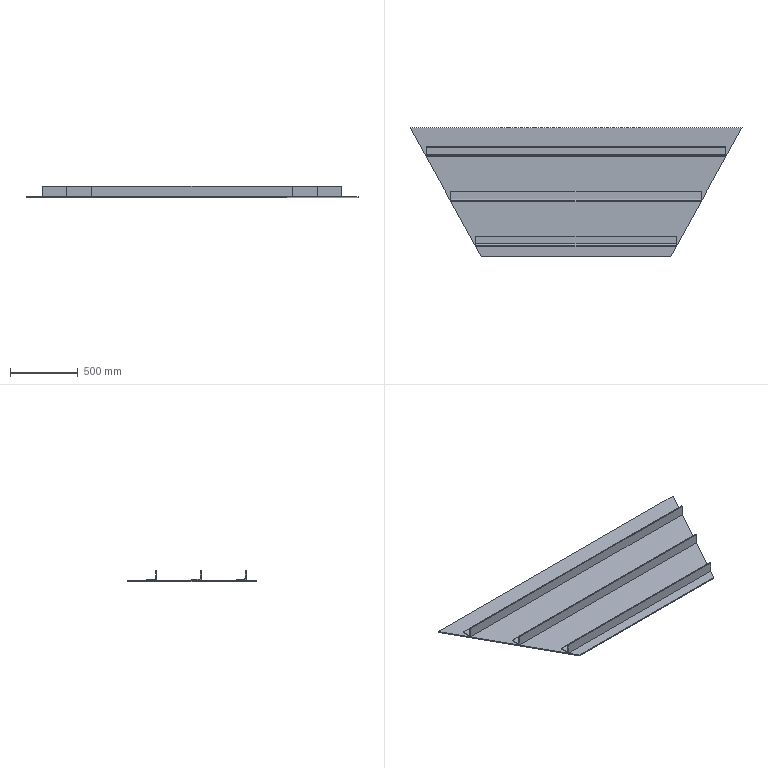Part | STEP file | Front baffle assembly 2_Default<As machined> | 4 solids | 39 faces | box 2450 x 950 x 83 mm | volume 21006283 mm3 | plane 30 | cylinder 9 | commonest cylinder face diameters 5.333 x6 18 x3